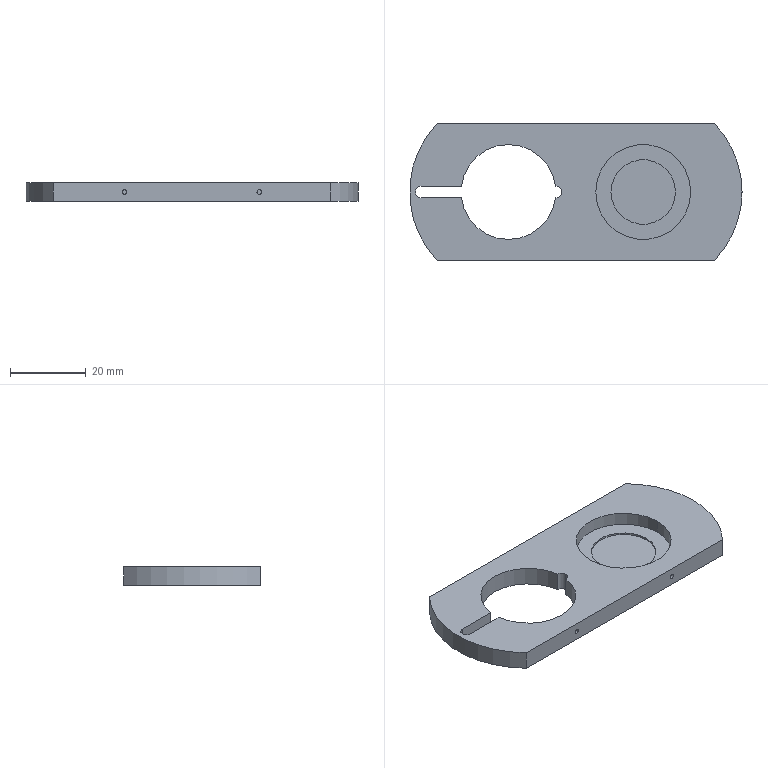Part | STEP file | TCHK-2D-D30-BB-2.stp.STEP | 1 solid | 28 faces | box 87.5 x 36 x 5 mm | volume 10454 mm3 | cylinder 16 | plane 12 | commonest cylinder face diameters 1.2 x4 25 x4 3 x3 52 x3 17 x2
STEP:
#1=CARTESIAN_POINT('',(-5.34,1.5,-2.5));
#2=VERTEX_POINT('',#1);
#3=CARTESIAN_POINT('',(-30.16,1.5,-2.5));
#4=VERTEX_POINT('',#3);
#5=CARTESIAN_POINT('',(-17.75,0.,-2.5));
#6=DIRECTION('',(0.,0.,1.));
#7=DIRECTION('',(0.9928,0.12,0.));
#8=AXIS2_PLACEMENT_3D('',#5,#6,#7);
#9=CIRCLE('',#8,12.5);
#10=EDGE_CURVE('',#2,#4,#9,.T.);
#11=ORIENTED_EDGE('',*,*,#10,.T.);
#12=CARTESIAN_POINT('',(-40.75,1.5,-2.5));
#13=VERTEX_POINT('',#12);
#14=CARTESIAN_POINT('',(-30.16,1.5,-2.5));
#15=DIRECTION('',(-1.,0.,0.));
#16=VECTOR('',#15,1000.);
#17=LINE('',#14,#16);
#18=EDGE_CURVE('',#4,#13,#17,.T.);
#19=ORIENTED_EDGE('',*,*,#18,.T.);
#20=CARTESIAN_POINT('',(-40.75,-1.5,-2.5));
#21=VERTEX_POINT('',#20);
#22=CARTESIAN_POINT('',(-40.75,0.,-2.5));
#23=DIRECTION('',(0.,0.,1.));
#24=DIRECTION('',(0.,1.,0.));
#25=AXIS2_PLACEMENT_3D('',#22,#23,#24);
#26=CIRCLE('',#25,1.5);
#27=EDGE_CURVE('',#13,#21,#26,.T.);
#28=ORIENTED_EDGE('',*,*,#27,.T.);
#29=CARTESIAN_POINT('',(-30.16,-1.5,-2.5));
#30=VERTEX_POINT('',#29);
#31=CARTESIAN_POINT('',(-40.75,-1.5,-2.5));
#32=DIRECTION('',(1.,0.,0.));
#33=VECTOR('',#32,1000.);
#34=LINE('',#31,#33);
#35=EDGE_CURVE('',#21,#30,#34,.T.);
#36=ORIENTED_EDGE('',*,*,#35,.T.);
#37=CARTESIAN_POINT('',(-5.34,-1.5,-2.5));
#38=VERTEX_POINT('',#37);
#39=CARTESIAN_POINT('',(-17.75,0.,-2.5));
#40=DIRECTION('',(0.,0.,1.));
#41=DIRECTION('',(-0.9928,-0.12,0.));
#42=AXIS2_PLACEMENT_3D('',#39,#40,#41);
#43=CIRCLE('',#42,12.5);
#44=EDGE_CURVE('',#30,#38,#43,.T.);
#45=ORIENTED_EDGE('',*,*,#44,.T.);
#46=CARTESIAN_POINT('',(-5.25,-1.5,-2.5));
#47=VERTEX_POINT('',#46);
#48=CARTESIAN_POINT('',(-5.34,-1.5,-2.5));
#49=DIRECTION('',(1.,0.,0.));
#50=VECTOR('',#49,1000.);
#51=LINE('',#48,#50);
#52=EDGE_CURVE('',#38,#47,#51,.T.);
#53=ORIENTED_EDGE('',*,*,#52,.T.);
#54=CARTESIAN_POINT('',(-3.75,0.,-2.5));
#55=VERTEX_POINT('',#54);
#56=CARTESIAN_POINT('',(-5.25,0.,-2.5));
#57=DIRECTION('',(0.,0.,1.));
#58=DIRECTION('',(0.,-1.,0.));
#59=AXIS2_PLACEMENT_3D('',#56,#57,#58);
#60=CIRCLE('',#59,1.5);
#61=EDGE_CURVE('',#47,#55,#60,.T.);
#62=ORIENTED_EDGE('',*,*,#61,.T.);
#63=CARTESIAN_POINT('',(-5.25,1.5,-2.5));
#64=VERTEX_POINT('',#63);
#65=CARTESIAN_POINT('',(-5.25,0.,-2.5));
#66=DIRECTION('',(0.,0.,1.));
#67=DIRECTION('',(0.,-1.,0.));
#68=AXIS2_PLACEMENT_3D('',#65,#66,#67);
#69=CIRCLE('',#68,1.5);
#70=EDGE_CURVE('',#55,#64,#69,.T.);
#71=ORIENTED_EDGE('',*,*,#70,.T.);
#72=CARTESIAN_POINT('',(-5.25,1.5,-2.5));
#73=DIRECTION('',(-1.,0.,0.));
#74=VECTOR('',#73,1000.);
#75=LINE('',#72,#74);
#76=EDGE_CURVE('',#64,#2,#75,.T.);
#77=ORIENTED_EDGE('',*,*,#76,.T.);
#78=EDGE_LOOP('',(#11,#19,#28,#36,#45,#53,#62,#71,#77));
#79=FACE_BOUND('',#78,.T.);
#80=CARTESIAN_POINT('',(36.512,18.,-2.5));
#81=VERTEX_POINT('',#80);
#82=CARTESIAN_POINT('',(-36.512,18.,-2.5));
#83=VERTEX_POINT('',#82);
#84=CARTESIAN_POINT('',(36.512,18.,-2.5));
#85=DIRECTION('',(-1.,0.,0.));
#86=VECTOR('',#85,1000.);
#87=LINE('',#84,#86);
#88=EDGE_CURVE('',#81,#83,#87,.T.);
#89=ORIENTED_EDGE('',*,*,#88,.F.);
#90=CARTESIAN_POINT('',(43.75,0.,-2.5));
#91=VERTEX_POINT('',#90);
#92=CARTESIAN_POINT('',(17.75,0.,-2.5));
#93=DIRECTION('',(0.,0.,1.));
#94=DIRECTION('',(0.7216,-0.6923,0.));
#95=AXIS2_PLACEMENT_3D('',#92,#93,#94);
#96=CIRCLE('',#95,26.);
#97=EDGE_CURVE('',#91,#81,#96,.T.);
#98=ORIENTED_EDGE('',*,*,#97,.F.);
#99=CARTESIAN_POINT('',(36.512,-18.,-2.5));
#100=VERTEX_POINT('',#99);
#101=CARTESIAN_POINT('',(17.75,0.,-2.5));
#102=DIRECTION('',(0.,0.,1.));
#103=DIRECTION('',(0.7216,-0.6923,0.));
#104=AXIS2_PLACEMENT_3D('',#101,#102,#103);
#105=CIRCLE('',#104,26.);
#106=EDGE_CURVE('',#100,#91,#105,.T.);
#107=ORIENTED_EDGE('',*,*,#106,.F.);
#108=CARTESIAN_POINT('',(-36.512,-18.,-2.5));
#109=VERTEX_POINT('',#108);
#110=CARTESIAN_POINT('',(-36.512,-18.,-2.5));
#111=DIRECTION('',(1.,0.,0.));
#112=VECTOR('',#111,1000.);
#113=LINE('',#110,#112);
#114=EDGE_CURVE('',#109,#100,#113,.T.);
#115=ORIENTED_EDGE('',*,*,#114,.F.);
#116=CARTESIAN_POINT('',(-17.75,0.,-2.5));
#117=DIRECTION('',(0.,0.,1.));
#118=DIRECTION('',(-0.7216,0.6923,0.));
#119=AXIS2_PLACEMENT_3D('',#116,#117,#118);
#120=CIRCLE('',#119,26.);
#121=EDGE_CURVE('',#83,#109,#120,.T.);
#122=ORIENTED_EDGE('',*,*,#121,.F.);
#123=EDGE_LOOP('',(#89,#98,#107,#115,#122));
#124=FACE_OUTER_BOUND('',#123,.T.);
#125=CARTESIAN_POINT('',(0.,0.,-2.5));
#126=DIRECTION('',(0.,0.,1.));
#127=DIRECTION('',(1.,0.,0.));
#128=AXIS2_PLACEMENT_3D('',#125,#126,#127);
#129=PLANE('',#128);
#130=ADVANCED_FACE('',(#79,#124),#129,.F.);
#131=CARTESIAN_POINT('',(-36.512,-18.,2.5));
#132=VERTEX_POINT('',#131);
#133=CARTESIAN_POINT('',(-36.512,-18.,-2.5));
#134=DIRECTION('',(0.,0.,1.));
#135=VECTOR('',#134,1000.);
#136=LINE('',#133,#135);
#137=EDGE_CURVE('',#109,#132,#136,.T.);
#138=ORIENTED_EDGE('',*,*,#137,.T.);
#139=CARTESIAN_POINT('',(-36.512,18.,2.5));
#140=VERTEX_POINT('',#139);
#141=CARTESIAN_POINT('',(-17.75,0.,2.5));
#142=DIRECTION('',(0.,0.,1.));
#143=DIRECTION('',(-0.7216,0.6923,0.));
#144=AXIS2_PLACEMENT_3D('',#141,#142,#143);
#145=CIRCLE('',#144,26.);
#146=EDGE_CURVE('',#140,#132,#145,.T.);
#147=ORIENTED_EDGE('',*,*,#146,.F.);
#148=CARTESIAN_POINT('',(-36.512,18.,-2.5));
#149=DIRECTION('',(0.,0.,1.));
#150=VECTOR('',#149,1000.);
#151=LINE('',#148,#150);
#152=EDGE_CURVE('',#83,#140,#151,.T.);
#153=ORIENTED_EDGE('',*,*,#152,.F.);
#154=ORIENTED_EDGE('',*,*,#121,.T.);
#155=EDGE_LOOP('',(#138,#147,#153,#154));
#156=FACE_OUTER_BOUND('',#155,.T.);
#157=CARTESIAN_POINT('',(-17.75,0.,-2.5));
#158=DIRECTION('',(0.,0.,1.));
#159=DIRECTION('',(1.,0.,0.));
#160=AXIS2_PLACEMENT_3D('',#157,#158,#159);
#161=CYLINDRICAL_SURFACE('',#160,26.);
#162=ADVANCED_FACE('',(#156),#161,.T.);
#163=ORIENTED_EDGE('',*,*,#152,.T.);
#164=CARTESIAN_POINT('',(36.512,18.,2.5));
#165=VERTEX_POINT('',#164);
#166=CARTESIAN_POINT('',(36.512,18.,2.5));
#167=DIRECTION('',(-1.,0.,0.));
#168=VECTOR('',#167,1000.);
#169=LINE('',#166,#168);
#170=EDGE_CURVE('',#165,#140,#169,.T.);
#171=ORIENTED_EDGE('',*,*,#170,.F.);
#172=CARTESIAN_POINT('',(36.512,18.,-2.5));
#173=DIRECTION('',(0.,0.,1.));
#174=VECTOR('',#173,1000.);
#175=LINE('',#172,#174);
#176=EDGE_CURVE('',#81,#165,#175,.T.);
#177=ORIENTED_EDGE('',*,*,#176,.F.);
#178=ORIENTED_EDGE('',*,*,#88,.T.);
#179=EDGE_LOOP('',(#163,#171,#177,#178));
#180=FACE_OUTER_BOUND('',#179,.T.);
#181=CARTESIAN_POINT('',(36.512,18.,-2.5));
#182=DIRECTION('',(0.,1.,0.));
#183=DIRECTION('',(1.,0.,0.));
#184=AXIS2_PLACEMENT_3D('',#181,#182,#183);
#185=PLANE('',#184);
#186=ADVANCED_FACE('',(#180),#185,.T.);
#187=CARTESIAN_POINT('',(43.75,0.,2.5));
#188=VERTEX_POINT('',#187);
#189=CARTESIAN_POINT('',(43.75,0.,-2.5));
#190=DIRECTION('',(0.,0.,1.));
#191=VECTOR('',#190,1000.);
#192=LINE('',#189,#191);
#193=EDGE_CURVE('',#91,#188,#192,.T.);
#194=ORIENTED_EDGE('',*,*,#193,.F.);
#195=ORIENTED_EDGE('',*,*,#97,.T.);
#196=ORIENTED_EDGE('',*,*,#176,.T.);
#197=CARTESIAN_POINT('',(17.75,0.,2.5));
#198=DIRECTION('',(0.,0.,1.));
#199=DIRECTION('',(0.7216,-0.6923,0.));
#200=AXIS2_PLACEMENT_3D('',#197,#198,#199);
#201=CIRCLE('',#200,26.);
#202=EDGE_CURVE('',#188,#165,#201,.T.);
#203=ORIENTED_EDGE('',*,*,#202,.F.);
#204=EDGE_LOOP('',(#194,#195,#196,#203));
#205=FACE_OUTER_BOUND('',#204,.T.);
#206=CARTESIAN_POINT('',(17.75,0.,-2.5));
#207=DIRECTION('',(0.,0.,1.));
#208=DIRECTION('',(1.,0.,0.));
#209=AXIS2_PLACEMENT_3D('',#206,#207,#208);
#210=CYLINDRICAL_SURFACE('',#209,26.);
#211=ADVANCED_FACE('',(#205),#210,.T.);
#212=CARTESIAN_POINT('',(-18.35,-18.,0.));
#213=VERTEX_POINT('',#212);
#214=CARTESIAN_POINT('',(-17.15,-18.,0.));
#215=VERTEX_POINT('',#214);
#216=CARTESIAN_POINT('',(-17.75,-18.,0.));
#217=DIRECTION('',(0.,1.,0.));
#218=DIRECTION('',(-1.,0.,0.));
#219=AXIS2_PLACEMENT_3D('',#216,#217,#218);
#220=CIRCLE('',#219,0.6);
#221=EDGE_CURVE('',#213,#215,#220,.T.);
#222=ORIENTED_EDGE('',*,*,#221,.T.);
#223=CARTESIAN_POINT('',(-17.75,-18.,0.));
#224=DIRECTION('',(0.,1.,0.));
#225=DIRECTION('',(1.,0.,0.));
#226=AXIS2_PLACEMENT_3D('',#223,#224,#225);
#227=CIRCLE('',#226,0.6);
#228=EDGE_CURVE('',#215,#213,#227,.T.);
#229=ORIENTED_EDGE('',*,*,#228,.T.);
#230=EDGE_LOOP('',(#222,#229));
#231=FACE_BOUND('',#230,.T.);
#232=CARTESIAN_POINT('',(17.15,-18.,0.));
#233=VERTEX_POINT('',#232);
#234=CARTESIAN_POINT('',(18.35,-18.,0.));
#235=VERTEX_POINT('',#234);
#236=CARTESIAN_POINT('',(17.75,-18.,0.));
#237=DIRECTION('',(0.,1.,0.));
#238=DIRECTION('',(-1.,0.,0.));
#239=AXIS2_PLACEMENT_3D('',#236,#237,#238);
#240=CIRCLE('',#239,0.6);
#241=EDGE_CURVE('',#233,#235,#240,.T.);
#242=ORIENTED_EDGE('',*,*,#241,.T.);
#243=CARTESIAN_POINT('',(17.75,-18.,0.));
#244=DIRECTION('',(0.,1.,0.));
#245=DIRECTION('',(1.,0.,0.));
#246=AXIS2_PLACEMENT_3D('',#243,#244,#245);
#247=CIRCLE('',#246,0.6);
#248=EDGE_CURVE('',#235,#233,#247,.T.);
#249=ORIENTED_EDGE('',*,*,#248,.T.);
#250=EDGE_LOOP('',(#242,#249));
#251=FACE_BOUND('',#250,.T.);
#252=CARTESIAN_POINT('',(36.512,-18.,2.5));
#253=VERTEX_POINT('',#252);
#254=CARTESIAN_POINT('',(36.512,-18.,-2.5));
#255=DIRECTION('',(0.,0.,1.));
#256=VECTOR('',#255,1000.);
#257=LINE('',#254,#256);
#258=EDGE_CURVE('',#100,#253,#257,.T.);
#259=ORIENTED_EDGE('',*,*,#258,.T.);
#260=CARTESIAN_POINT('',(-36.512,-18.,2.5));
#261=DIRECTION('',(1.,0.,0.));
#262=VECTOR('',#261,1000.);
#263=LINE('',#260,#262);
#264=EDGE_CURVE('',#132,#253,#263,.T.);
#265=ORIENTED_EDGE('',*,*,#264,.F.);
#266=ORIENTED_EDGE('',*,*,#137,.F.);
#267=ORIENTED_EDGE('',*,*,#114,.T.);
#268=EDGE_LOOP('',(#259,#265,#266,#267));
#269=FACE_OUTER_BOUND('',#268,.T.);
#270=CARTESIAN_POINT('',(-36.512,-18.,-2.5));
#271=DIRECTION('',(0.,-1.,0.));
#272=DIRECTION('',(0.,0.,-1.));
#273=AXIS2_PLACEMENT_3D('',#270,#271,#272);
#274=PLANE('',#273);
#275=ADVANCED_FACE('',(#231,#251,#269),#274,.T.);
#276=CARTESIAN_POINT('',(5.25,0.,2.5));
#277=VERTEX_POINT('',#276);
#278=CARTESIAN_POINT('',(30.25,0.,2.5));
#279=VERTEX_POINT('',#278);
#280=CARTESIAN_POINT('',(17.75,0.,2.5));
#281=DIRECTION('',(0.,0.,1.));
#282=DIRECTION('',(-1.,0.,0.));
#283=AXIS2_PLACEMENT_3D('',#280,#281,#282);
#284=CIRCLE('',#283,12.5);
#285=EDGE_CURVE('',#277,#279,#284,.T.);
#286=ORIENTED_EDGE('',*,*,#285,.F.);
#287=CARTESIAN_POINT('',(17.75,0.,2.5));
#288=DIRECTION('',(0.,0.,1.));
#289=DIRECTION('',(1.,0.,0.));
#290=AXIS2_PLACEMENT_3D('',#287,#288,#289);
#291=CIRCLE('',#290,12.5);
#292=EDGE_CURVE('',#279,#277,#291,.T.);
#293=ORIENTED_EDGE('',*,*,#292,.F.);
#294=EDGE_LOOP('',(#286,#293));
#295=FACE_BOUND('',#294,.T.);
#296=CARTESIAN_POINT('',(-5.25,-1.5,2.5));
#297=VERTEX_POINT('',#296);
#298=CARTESIAN_POINT('',(-3.75,0.,2.5));
#299=VERTEX_POINT('',#298);
#300=CARTESIAN_POINT('',(-5.25,0.,2.5));
#301=DIRECTION('',(0.,0.,1.));
#302=DIRECTION('',(0.,-1.,0.));
#303=AXIS2_PLACEMENT_3D('',#300,#301,#302);
#304=CIRCLE('',#303,1.5);
#305=EDGE_CURVE('',#297,#299,#304,.T.);
#306=ORIENTED_EDGE('',*,*,#305,.F.);
#307=CARTESIAN_POINT('',(-5.34,-1.5,2.5));
#308=VERTEX_POINT('',#307);
#309=CARTESIAN_POINT('',(-5.34,-1.5,2.5));
#310=DIRECTION('',(1.,0.,0.));
#311=VECTOR('',#310,1000.);
#312=LINE('',#309,#311);
#313=EDGE_CURVE('',#308,#297,#312,.T.);
#314=ORIENTED_EDGE('',*,*,#313,.F.);
#315=CARTESIAN_POINT('',(-30.16,-1.5,2.5));
#316=VERTEX_POINT('',#315);
#317=CARTESIAN_POINT('',(-17.75,0.,2.5));
#318=DIRECTION('',(0.,0.,1.));
#319=DIRECTION('',(-0.9928,-0.12,0.));
#320=AXIS2_PLACEMENT_3D('',#317,#318,#319);
#321=CIRCLE('',#320,12.5);
#322=EDGE_CURVE('',#316,#308,#321,.T.);
#323=ORIENTED_EDGE('',*,*,#322,.F.);
#324=CARTESIAN_POINT('',(-40.75,-1.5,2.5));
#325=VERTEX_POINT('',#324);
#326=CARTESIAN_POINT('',(-40.75,-1.5,2.5));
#327=DIRECTION('',(1.,0.,0.));
#328=VECTOR('',#327,1000.);
#329=LINE('',#326,#328);
#330=EDGE_CURVE('',#325,#316,#329,.T.);
#331=ORIENTED_EDGE('',*,*,#330,.F.);
#332=CARTESIAN_POINT('',(-40.75,1.5,2.5));
#333=VERTEX_POINT('',#332);
#334=CARTESIAN_POINT('',(-40.75,0.,2.5));
#335=DIRECTION('',(0.,0.,1.));
#336=DIRECTION('',(0.,1.,0.));
#337=AXIS2_PLACEMENT_3D('',#334,#335,#336);
#338=CIRCLE('',#337,1.5);
#339=EDGE_CURVE('',#333,#325,#338,.T.);
#340=ORIENTED_EDGE('',*,*,#339,.F.);
#341=CARTESIAN_POINT('',(-30.16,1.5,2.5));
#342=VERTEX_POINT('',#341);
#343=CARTESIAN_POINT('',(-30.16,1.5,2.5));
#344=DIRECTION('',(-1.,0.,0.));
#345=VECTOR('',#344,1000.);
#346=LINE('',#343,#345);
#347=EDGE_CURVE('',#342,#333,#346,.T.);
#348=ORIENTED_EDGE('',*,*,#347,.F.);
#349=CARTESIAN_POINT('',(-5.34,1.5,2.5));
#350=VERTEX_POINT('',#349);
#351=CARTESIAN_POINT('',(-17.75,0.,2.5));
#352=DIRECTION('',(0.,0.,1.));
#353=DIRECTION('',(0.9928,0.12,0.));
#354=AXIS2_PLACEMENT_3D('',#351,#352,#353);
#355=CIRCLE('',#354,12.5);
#356=EDGE_CURVE('',#350,#342,#355,.T.);
#357=ORIENTED_EDGE('',*,*,#356,.F.);
#358=CARTESIAN_POINT('',(-5.25,1.5,2.5));
#359=VERTEX_POINT('',#358);
#360=CARTESIAN_POINT('',(-5.25,1.5,2.5));
#361=DIRECTION('',(-1.,0.,0.));
#362=VECTOR('',#361,1000.);
#363=LINE('',#360,#362);
#364=EDGE_CURVE('',#359,#350,#363,.T.);
#365=ORIENTED_EDGE('',*,*,#364,.F.);
#366=CARTESIAN_POINT('',(-5.25,0.,2.5));
#367=DIRECTION('',(0.,0.,1.));
#368=DIRECTION('',(0.,-1.,0.));
#369=AXIS2_PLACEMENT_3D('',#366,#367,#368);
#370=CIRCLE('',#369,1.5);
#371=EDGE_CURVE('',#299,#359,#370,.T.);
#372=ORIENTED_EDGE('',*,*,#371,.F.);
#373=EDGE_LOOP('',(#306,#314,#323,#331,#340,#348,#357,#365,#372));
#374=FACE_BOUND('',#373,.T.);
#375=ORIENTED_EDGE('',*,*,#264,.T.);
#376=CARTESIAN_POINT('',(17.75,0.,2.5));
#377=DIRECTION('',(0.,0.,1.));
#378=DIRECTION('',(0.7216,-0.6923,0.));
#379=AXIS2_PLACEMENT_3D('',#376,#377,#378);
#380=CIRCLE('',#379,26.);
#381=EDGE_CURVE('',#253,#188,#380,.T.);
#382=ORIENTED_EDGE('',*,*,#381,.T.);
#383=ORIENTED_EDGE('',*,*,#202,.T.);
#384=ORIENTED_EDGE('',*,*,#170,.T.);
#385=ORIENTED_EDGE('',*,*,#146,.T.);
#386=EDGE_LOOP('',(#375,#382,#383,#384,#385));
#387=FACE_OUTER_BOUND('',#386,.T.);
#388=CARTESIAN_POINT('',(0.,0.,2.5));
#389=DIRECTION('',(0.,0.,1.));
#390=DIRECTION('',(1.,0.,0.));
#391=AXIS2_PLACEMENT_3D('',#388,#389,#390);
#392=PLANE('',#391);
#393=ADVANCED_FACE('',(#295,#374,#387),#392,.T.);
#394=CARTESIAN_POINT('',(5.25,0.,-1.));
#395=VERTEX_POINT('',#394);
#396=CARTESIAN_POINT('',(5.25,0.,2.5));
#397=DIRECTION('',(0.,0.,-1.));
#398=VECTOR('',#397,1000.);
#399=LINE('',#396,#398);
#400=EDGE_CURVE('',#277,#395,#399,.T.);
#401=ORIENTED_EDGE('',*,*,#400,.T.);
#402=CARTESIAN_POINT('',(30.25,0.,-1.));
#403=VERTEX_POINT('',#402);
#404=CARTESIAN_POINT('',(17.75,0.,-1.));
#405=DIRECTION('',(0.,0.,-1.));
#406=DIRECTION('',(-1.,0.,0.));
#407=AXIS2_PLACEMENT_3D('',#404,#405,#406);
#408=CIRCLE('',#407,12.5);
#409=EDGE_CURVE('',#395,#403,#408,.T.);
#410=ORIENTED_EDGE('',*,*,#409,.T.);
#411=CARTESIAN_POINT('',(30.25,0.,2.5));
#412=DIRECTION('',(0.,0.,-1.));
#413=VECTOR('',#412,1000.);
#414=LINE('',#411,#413);
#415=EDGE_CURVE('',#279,#403,#414,.T.);
#416=ORIENTED_EDGE('',*,*,#415,.F.);
#417=ORIENTED_EDGE('',*,*,#292,.T.);
#418=EDGE_LOOP('',(#401,#410,#416,#417));
#419=FACE_OUTER_BOUND('',#418,.T.);
#420=CARTESIAN_POINT('',(17.75,0.,2.5));
#421=DIRECTION('',(0.,0.,1.));
#422=DIRECTION('',(1.,0.,0.));
#423=AXIS2_PLACEMENT_3D('',#420,#421,#422);
#424=CYLINDRICAL_SURFACE('',#423,12.5);
#425=ADVANCED_FACE('',(#419),#424,.F.);
#426=ORIENTED_EDGE('',*,*,#415,.T.);
#427=CARTESIAN_POINT('',(17.75,0.,-1.));
#428=DIRECTION('',(0.,0.,-1.));
#429=DIRECTION('',(1.,0.,0.));
#430=AXIS2_PLACEMENT_3D('',#427,#428,#429);
#431=CIRCLE('',#430,12.5);
#432=EDGE_CURVE('',#403,#395,#431,.T.);
#433=ORIENTED_EDGE('',*,*,#432,.T.);
#434=ORIENTED_EDGE('',*,*,#400,.F.);
#435=ORIENTED_EDGE('',*,*,#285,.T.);
#436=EDGE_LOOP('',(#426,#433,#434,#435));
#437=FACE_OUTER_BOUND('',#436,.T.);
#438=CARTESIAN_POINT('',(17.75,0.,2.5));
#439=DIRECTION('',(0.,0.,1.));
#440=DIRECTION('',(1.,0.,0.));
#441=AXIS2_PLACEMENT_3D('',#438,#439,#440);
#442=CYLINDRICAL_SURFACE('',#441,12.5);
#443=ADVANCED_FACE('',(#437),#442,.F.);
#444=CARTESIAN_POINT('',(9.25,0.,-1.));
#445=VERTEX_POINT('',#444);
#446=CARTESIAN_POINT('',(26.25,0.,-1.));
#447=VERTEX_POINT('',#446);
#448=CARTESIAN_POINT('',(17.75,0.,-1.));
#449=DIRECTION('',(0.,0.,1.));
#450=DIRECTION('',(-1.,0.,0.));
#451=AXIS2_PLACEMENT_3D('',#448,#449,#450);
#452=CIRCLE('',#451,8.5);
#453=EDGE_CURVE('',#445,#447,#452,.T.);
#454=ORIENTED_EDGE('',*,*,#453,.F.);
#455=CARTESIAN_POINT('',(17.75,0.,-1.));
#456=DIRECTION('',(0.,0.,1.));
#457=DIRECTION('',(1.,0.,0.));
#458=AXIS2_PLACEMENT_3D('',#455,#456,#457);
#459=CIRCLE('',#458,8.5);
#460=EDGE_CURVE('',#447,#445,#459,.T.);
#461=ORIENTED_EDGE('',*,*,#460,.F.);
#462=EDGE_LOOP('',(#454,#461));
#463=FACE_BOUND('',#462,.T.);
#464=ORIENTED_EDGE('',*,*,#432,.F.);
#465=ORIENTED_EDGE('',*,*,#409,.F.);
#466=EDGE_LOOP('',(#464,#465));
#467=FACE_OUTER_BOUND('',#466,.T.);
#468=CARTESIAN_POINT('',(0.,0.,-1.));
#469=DIRECTION('',(0.,0.,1.));
#470=DIRECTION('',(1.,0.,0.));
#471=AXIS2_PLACEMENT_3D('',#468,#469,#470);
#472=PLANE('',#471);
#473=ADVANCED_FACE('',(#463,#467),#472,.T.);
#474=CARTESIAN_POINT('',(9.25,0.,-1.5));
#475=VERTEX_POINT('',#474);
#476=CARTESIAN_POINT('',(9.25,0.,-1.));
#477=DIRECTION('',(0.,0.,-1.));
#478=VECTOR('',#477,1000.);
#479=LINE('',#476,#478);
#480=EDGE_CURVE('',#445,#475,#479,.T.);
#481=ORIENTED_EDGE('',*,*,#480,.T.);
#482=CARTESIAN_POINT('',(26.25,0.,-1.5));
#483=VERTEX_POINT('',#482);
#484=CARTESIAN_POINT('',(17.75,0.,-1.5));
#485=DIRECTION('',(0.,0.,1.));
#486=DIRECTION('',(1.,0.,0.));
#487=AXIS2_PLACEMENT_3D('',#484,#485,#486);
#488=CIRCLE('',#487,8.5);
#489=EDGE_CURVE('',#483,#475,#488,.T.);
#490=ORIENTED_EDGE('',*,*,#489,.F.);
#491=CARTESIAN_POINT('',(26.25,0.,-1.));
#492=DIRECTION('',(0.,0.,-1.));
#493=VECTOR('',#492,1000.);
#494=LINE('',#491,#493);
#495=EDGE_CURVE('',#447,#483,#494,.T.);
#496=ORIENTED_EDGE('',*,*,#495,.F.);
#497=ORIENTED_EDGE('',*,*,#460,.T.);
#498=EDGE_LOOP('',(#481,#490,#496,#497));
#499=FACE_OUTER_BOUND('',#498,.T.);
#500=CARTESIAN_POINT('',(17.75,0.,-1.));
#501=DIRECTION('',(0.,0.,1.));
#502=DIRECTION('',(1.,0.,0.));
#503=AXIS2_PLACEMENT_3D('',#500,#501,#502);
#504=CYLINDRICAL_SURFACE('',#503,8.5);
#505=ADVANCED_FACE('',(#499),#504,.F.);
#506=ORIENTED_EDGE('',*,*,#495,.T.);
#507=CARTESIAN_POINT('',(17.75,0.,-1.5));
#508=DIRECTION('',(0.,0.,1.));
#509=DIRECTION('',(-1.,0.,0.));
#510=AXIS2_PLACEMENT_3D('',#507,#508,#509);
#511=CIRCLE('',#510,8.5);
#512=EDGE_CURVE('',#475,#483,#511,.T.);
#513=ORIENTED_EDGE('',*,*,#512,.F.);
#514=ORIENTED_EDGE('',*,*,#480,.F.);
#515=ORIENTED_EDGE('',*,*,#453,.T.);
#516=EDGE_LOOP('',(#506,#513,#514,#515));
#517=FACE_OUTER_BOUND('',#516,.T.);
#518=CARTESIAN_POINT('',(17.75,0.,-1.));
#519=DIRECTION('',(0.,0.,1.));
#520=DIRECTION('',(1.,0.,0.));
#521=AXIS2_PLACEMENT_3D('',#518,#519,#520);
#522=CYLINDRICAL_SURFACE('',#521,8.5);
#523=ADVANCED_FACE('',(#517),#522,.F.);
#524=ORIENTED_EDGE('',*,*,#512,.T.);
#525=ORIENTED_EDGE('',*,*,#489,.T.);
#526=EDGE_LOOP('',(#524,#525));
#527=FACE_OUTER_BOUND('',#526,.T.);
#528=CARTESIAN_POINT('',(0.,0.,-1.5));
#529=DIRECTION('',(0.,0.,1.));
#530=DIRECTION('',(1.,0.,0.));
#531=AXIS2_PLACEMENT_3D('',#528,#529,#530);
#532=PLANE('',#531);
#533=ADVANCED_FACE('',(#527),#532,.T.);
#534=CARTESIAN_POINT('',(-5.25,1.5,2.5));
#535=DIRECTION('',(0.,0.,-1.));
#536=VECTOR('',#535,1000.);
#537=LINE('',#534,#536);
#538=EDGE_CURVE('',#359,#64,#537,.T.);
#539=ORIENTED_EDGE('',*,*,#538,.F.);
#540=ORIENTED_EDGE('',*,*,#364,.T.);
#541=CARTESIAN_POINT('',(-5.34,1.5,-2.5));
#542=DIRECTION('',(0.,0.,1.));
#543=VECTOR('',#542,1000.);
#544=LINE('',#541,#543);
#545=EDGE_CURVE('',#2,#350,#544,.T.);
#546=ORIENTED_EDGE('',*,*,#545,.F.);
#547=ORIENTED_EDGE('',*,*,#76,.F.);
#548=EDGE_LOOP('',(#539,#540,#546,#547));
#549=FACE_OUTER_BOUND('',#548,.T.);
#550=CARTESIAN_POINT('',(-5.25,1.5,2.5));
#551=DIRECTION('',(0.,1.,0.));
#552=DIRECTION('',(1.,0.,0.));
#553=AXIS2_PLACEMENT_3D('',#550,#551,#552);
#554=PLANE('',#553);
#555=ADVANCED_FACE('',(#549),#554,.F.);
#556=CARTESIAN_POINT('',(-30.16,1.5,-2.5));
#557=DIRECTION('',(0.,0.,1.));
#558=VECTOR('',#557,1000.);
#559=LINE('',#556,#558);
#560=EDGE_CURVE('',#4,#342,#559,.T.);
#561=ORIENTED_EDGE('',*,*,#560,.T.);
#562=ORIENTED_EDGE('',*,*,#347,.T.);
#563=CARTESIAN_POINT('',(-40.75,1.5,2.5));
#564=DIRECTION('',(0.,0.,-1.));
#565=VECTOR('',#564,1000.);
#566=LINE('',#563,#565);
#567=EDGE_CURVE('',#333,#13,#566,.T.);
#568=ORIENTED_EDGE('',*,*,#567,.T.);
#569=ORIENTED_EDGE('',*,*,#18,.F.);
#570=EDGE_LOOP('',(#561,#562,#568,#569));
#571=FACE_OUTER_BOUND('',#570,.T.);
#572=CARTESIAN_POINT('',(-5.25,1.5,2.5));
#573=DIRECTION('',(0.,1.,0.));
#574=DIRECTION('',(1.,0.,0.));
#575=AXIS2_PLACEMENT_3D('',#572,#573,#574);
#576=PLANE('',#575);
#577=ADVANCED_FACE('',(#571),#576,.F.);
#578=ORIENTED_EDGE('',*,*,#356,.T.);
#579=ORIENTED_EDGE('',*,*,#560,.F.);
#580=ORIENTED_EDGE('',*,*,#10,.F.);
#581=ORIENTED_EDGE('',*,*,#545,.T.);
#582=EDGE_LOOP('',(#578,#579,#580,#581));
#583=FACE_OUTER_BOUND('',#582,.T.);
#584=CARTESIAN_POINT('',(-17.75,0.,2.5));
#585=DIRECTION('',(0.,0.,1.));
#586=DIRECTION('',(1.,0.,0.));
#587=AXIS2_PLACEMENT_3D('',#584,#585,#586);
#588=CYLINDRICAL_SURFACE('',#587,12.5);
#589=ADVANCED_FACE('',(#583),#588,.F.);
#590=CARTESIAN_POINT('',(-3.75,0.,2.5));
#591=DIRECTION('',(0.,0.,1.));
#592=VECTOR('',#591,1000.);
#593=LINE('',#590,#592);
#594=EDGE_CURVE('',#55,#299,#593,.T.);
#595=ORIENTED_EDGE('',*,*,#594,.F.);
#596=ORIENTED_EDGE('',*,*,#61,.F.);
#597=CARTESIAN_POINT('',(-5.25,-1.5,2.5));
#598=DIRECTION('',(0.,0.,-1.));
#599=VECTOR('',#598,1000.);
#600=LINE('',#597,#599);
#601=EDGE_CURVE('',#297,#47,#600,.T.);
#602=ORIENTED_EDGE('',*,*,#601,.F.);
#603=ORIENTED_EDGE('',*,*,#305,.T.);
#604=EDGE_LOOP('',(#595,#596,#602,#603));
#605=FACE_OUTER_BOUND('',#604,.T.);
#606=CARTESIAN_POINT('',(-5.25,0.,2.5));
#607=DIRECTION('',(0.,0.,1.));
#608=DIRECTION('',(1.,0.,0.));
#609=AXIS2_PLACEMENT_3D('',#606,#607,#608);
#610=CYLINDRICAL_SURFACE('',#609,1.5);
#611=ADVANCED_FACE('',(#605),#610,.F.);
#612=CARTESIAN_POINT('',(-40.75,-1.5,2.5));
#613=DIRECTION('',(0.,0.,-1.));
#614=VECTOR('',#613,1000.);
#615=LINE('',#612,#614);
#616=EDGE_CURVE('',#325,#21,#615,.T.);
#617=ORIENTED_EDGE('',*,*,#616,.F.);
#618=ORIENTED_EDGE('',*,*,#330,.T.);
#619=CARTESIAN_POINT('',(-30.16,-1.5,-2.5));
#620=DIRECTION('',(0.,0.,1.));
#621=VECTOR('',#620,1000.);
#622=LINE('',#619,#621);
#623=EDGE_CURVE('',#30,#316,#622,.T.);
#624=ORIENTED_EDGE('',*,*,#623,.F.);
#625=ORIENTED_EDGE('',*,*,#35,.F.);
#626=EDGE_LOOP('',(#617,#618,#624,#625));
#627=FACE_OUTER_BOUND('',#626,.T.);
#628=CARTESIAN_POINT('',(-40.75,-1.5,2.5));
#629=DIRECTION('',(0.,-1.,0.));
#630=DIRECTION('',(0.,0.,-1.));
#631=AXIS2_PLACEMENT_3D('',#628,#629,#630);
#632=PLANE('',#631);
#633=ADVANCED_FACE('',(#627),#632,.F.);
#634=CARTESIAN_POINT('',(-5.34,-1.5,-2.5));
#635=DIRECTION('',(0.,0.,1.));
#636=VECTOR('',#635,1000.);
#637=LINE('',#634,#636);
#638=EDGE_CURVE('',#38,#308,#637,.T.);
#639=ORIENTED_EDGE('',*,*,#638,.T.);
#640=ORIENTED_EDGE('',*,*,#313,.T.);
#641=ORIENTED_EDGE('',*,*,#601,.T.);
#642=ORIENTED_EDGE('',*,*,#52,.F.);
#643=EDGE_LOOP('',(#639,#640,#641,#642));
#644=FACE_OUTER_BOUND('',#643,.T.);
#645=CARTESIAN_POINT('',(-40.75,-1.5,2.5));
#646=DIRECTION('',(0.,-1.,0.));
#647=DIRECTION('',(0.,0.,-1.));
#648=AXIS2_PLACEMENT_3D('',#645,#646,#647);
#649=PLANE('',#648);
#650=ADVANCED_FACE('',(#644),#649,.F.);
#651=ORIENTED_EDGE('',*,*,#322,.T.);
#652=ORIENTED_EDGE('',*,*,#638,.F.);
#653=ORIENTED_EDGE('',*,*,#44,.F.);
#654=ORIENTED_EDGE('',*,*,#623,.T.);
#655=EDGE_LOOP('',(#651,#652,#653,#654));
#656=FACE_OUTER_BOUND('',#655,.T.);
#657=CARTESIAN_POINT('',(-17.75,0.,2.5));
#658=DIRECTION('',(0.,0.,1.));
#659=DIRECTION('',(1.,0.,0.));
#660=AXIS2_PLACEMENT_3D('',#657,#658,#659);
#661=CYLINDRICAL_SURFACE('',#660,12.5);
#662=ADVANCED_FACE('',(#656),#661,.F.);
#663=ORIENTED_EDGE('',*,*,#567,.F.);
#664=ORIENTED_EDGE('',*,*,#339,.T.);
#665=ORIENTED_EDGE('',*,*,#616,.T.);
#666=ORIENTED_EDGE('',*,*,#27,.F.);
#667=EDGE_LOOP('',(#663,#664,#665,#666));
#668=FACE_OUTER_BOUND('',#667,.T.);
#669=CARTESIAN_POINT('',(-40.75,0.,2.5));
#670=DIRECTION('',(0.,0.,1.));
#671=DIRECTION('',(1.,0.,0.));
#672=AXIS2_PLACEMENT_3D('',#669,#670,#671);
#673=CYLINDRICAL_SURFACE('',#672,1.5);
#674=ADVANCED_FACE('',(#668),#673,.F.);
#675=CARTESIAN_POINT('',(-17.15,-16.8,0.));
#676=VERTEX_POINT('',#675);
#677=CARTESIAN_POINT('',(-17.15,-18.,0.));
#678=DIRECTION('',(0.,1.,0.));
#679=VECTOR('',#678,1000.);
#680=LINE('',#677,#679);
#681=EDGE_CURVE('',#215,#676,#680,.T.);
#682=ORIENTED_EDGE('',*,*,#681,.T.);
#683=CARTESIAN_POINT('',(-18.35,-16.8,0.));
#684=VERTEX_POINT('',#683);
#685=CARTESIAN_POINT('',(-17.75,-16.8,0.));
#686=DIRECTION('',(0.,1.,0.));
#687=DIRECTION('',(1.,0.,0.));
#688=AXIS2_PLACEMENT_3D('',#685,#686,#687);
#689=CIRCLE('',#688,0.6);
#690=EDGE_CURVE('',#676,#684,#689,.T.);
#691=ORIENTED_EDGE('',*,*,#690,.T.);
#692=CARTESIAN_POINT('',(-18.35,-18.,0.));
#693=DIRECTION('',(0.,1.,0.));
#694=VECTOR('',#693,1000.);
#695=LINE('',#692,#694);
#696=EDGE_CURVE('',#213,#684,#695,.T.);
#697=ORIENTED_EDGE('',*,*,#696,.F.);
#698=ORIENTED_EDGE('',*,*,#228,.F.);
#699=EDGE_LOOP('',(#682,#691,#697,#698));
#700=FACE_OUTER_BOUND('',#699,.T.);
#701=CARTESIAN_POINT('',(-17.75,-18.,0.));
#702=DIRECTION('',(0.,1.,0.));
#703=DIRECTION('',(1.,0.,0.));
#704=AXIS2_PLACEMENT_3D('',#701,#702,#703);
#705=CYLINDRICAL_SURFACE('',#704,0.6);
#706=ADVANCED_FACE('',(#700),#705,.F.);
#707=ORIENTED_EDGE('',*,*,#696,.T.);
#708=CARTESIAN_POINT('',(-17.75,-16.8,0.));
#709=DIRECTION('',(0.,1.,0.));
#710=DIRECTION('',(-1.,0.,0.));
#711=AXIS2_PLACEMENT_3D('',#708,#709,#710);
#712=CIRCLE('',#711,0.6);
#713=EDGE_CURVE('',#684,#676,#712,.T.);
#714=ORIENTED_EDGE('',*,*,#713,.T.);
#715=ORIENTED_EDGE('',*,*,#681,.F.);
#716=ORIENTED_EDGE('',*,*,#221,.F.);
#717=EDGE_LOOP('',(#707,#714,#715,#716));
#718=FACE_OUTER_BOUND('',#717,.T.);
#719=CARTESIAN_POINT('',(-17.75,-18.,0.));
#720=DIRECTION('',(0.,1.,0.));
#721=DIRECTION('',(1.,0.,0.));
#722=AXIS2_PLACEMENT_3D('',#719,#720,#721);
#723=CYLINDRICAL_SURFACE('',#722,0.6);
#724=ADVANCED_FACE('',(#718),#723,.F.);
#725=ORIENTED_EDGE('',*,*,#713,.F.);
#726=ORIENTED_EDGE('',*,*,#690,.F.);
#727=EDGE_LOOP('',(#725,#726));
#728=FACE_OUTER_BOUND('',#727,.T.);
#729=CARTESIAN_POINT('',(0.,-16.8,-2.5));
#730=DIRECTION('',(0.,1.,0.));
#731=DIRECTION('',(1.,0.,0.));
#732=AXIS2_PLACEMENT_3D('',#729,#730,#731);
#733=PLANE('',#732);
#734=ADVANCED_FACE('',(#728),#733,.F.);
#735=CARTESIAN_POINT('',(17.15,-16.8,0.));
#736=VERTEX_POINT('',#735);
#737=CARTESIAN_POINT('',(18.35,-16.8,0.));
#738=VERTEX_POINT('',#737);
#739=CARTESIAN_POINT('',(17.75,-16.8,0.));
#740=DIRECTION('',(0.,1.,0.));
#741=DIRECTION('',(-1.,0.,0.));
#742=AXIS2_PLACEMENT_3D('',#739,#740,#741);
#743=CIRCLE('',#742,0.6);
#744=EDGE_CURVE('',#736,#738,#743,.T.);
#745=ORIENTED_EDGE('',*,*,#744,.F.);
#746=CARTESIAN_POINT('',(17.75,-16.8,0.));
#747=DIRECTION('',(0.,1.,0.));
#748=DIRECTION('',(1.,0.,0.));
#749=AXIS2_PLACEMENT_3D('',#746,#747,#748);
#750=CIRCLE('',#749,0.6);
#751=EDGE_CURVE('',#738,#736,#750,.T.);
#752=ORIENTED_EDGE('',*,*,#751,.F.);
#753=EDGE_LOOP('',(#745,#752));
#754=FACE_OUTER_BOUND('',#753,.T.);
#755=CARTESIAN_POINT('',(0.,-16.8,-2.5));
#756=DIRECTION('',(0.,1.,0.));
#757=DIRECTION('',(1.,0.,0.));
#758=AXIS2_PLACEMENT_3D('',#755,#756,#757);
#759=PLANE('',#758);
#760=ADVANCED_FACE('',(#754),#759,.F.);
#761=CARTESIAN_POINT('',(18.35,-18.,0.));
#762=DIRECTION('',(0.,1.,0.));
#763=VECTOR('',#762,1000.);
#764=LINE('',#761,#763);
#765=EDGE_CURVE('',#235,#738,#764,.T.);
#766=ORIENTED_EDGE('',*,*,#765,.T.);
#767=ORIENTED_EDGE('',*,*,#751,.T.);
#768=CARTESIAN_POINT('',(17.15,-18.,0.));
#769=DIRECTION('',(0.,1.,0.));
#770=VECTOR('',#769,1000.);
#771=LINE('',#768,#770);
#772=EDGE_CURVE('',#233,#736,#771,.T.);
#773=ORIENTED_EDGE('',*,*,#772,.F.);
#774=ORIENTED_EDGE('',*,*,#248,.F.);
#775=EDGE_LOOP('',(#766,#767,#773,#774));
#776=FACE_OUTER_BOUND('',#775,.T.);
#777=CARTESIAN_POINT('',(17.75,-18.,0.));
#778=DIRECTION('',(0.,1.,0.));
#779=DIRECTION('',(1.,0.,0.));
#780=AXIS2_PLACEMENT_3D('',#777,#778,#779);
#781=CYLINDRICAL_SURFACE('',#780,0.6);
#782=ADVANCED_FACE('',(#776),#781,.F.);
#783=ORIENTED_EDGE('',*,*,#772,.T.);
#784=ORIENTED_EDGE('',*,*,#744,.T.);
#785=ORIENTED_EDGE('',*,*,#765,.F.);
#786=ORIENTED_EDGE('',*,*,#241,.F.);
#787=EDGE_LOOP('',(#783,#784,#785,#786));
#788=FACE_OUTER_BOUND('',#787,.T.);
#789=CARTESIAN_POINT('',(17.75,-18.,0.));
#790=DIRECTION('',(0.,1.,0.));
#791=DIRECTION('',(1.,0.,0.));
#792=AXIS2_PLACEMENT_3D('',#789,#790,#791);
#793=CYLINDRICAL_SURFACE('',#792,0.6);
#794=ADVANCED_FACE('',(#788),#793,.F.);
#795=ORIENTED_EDGE('',*,*,#70,.F.);
#796=ORIENTED_EDGE('',*,*,#594,.T.);
#797=ORIENTED_EDGE('',*,*,#371,.T.);
#798=ORIENTED_EDGE('',*,*,#538,.T.);
#799=EDGE_LOOP('',(#795,#796,#797,#798));
#800=FACE_OUTER_BOUND('',#799,.T.);
#801=CARTESIAN_POINT('',(-5.25,0.,2.5));
#802=DIRECTION('',(0.,0.,1.));
#803=DIRECTION('',(1.,0.,0.));
#804=AXIS2_PLACEMENT_3D('',#801,#802,#803);
#805=CYLINDRICAL_SURFACE('',#804,1.5);
#806=ADVANCED_FACE('',(#800),#805,.F.);
#807=ORIENTED_EDGE('',*,*,#106,.T.);
#808=ORIENTED_EDGE('',*,*,#193,.T.);
#809=ORIENTED_EDGE('',*,*,#381,.F.);
#810=ORIENTED_EDGE('',*,*,#258,.F.);
#811=EDGE_LOOP('',(#807,#808,#809,#810));
#812=FACE_OUTER_BOUND('',#811,.T.);
#813=CARTESIAN_POINT('',(17.75,0.,-2.5));
#814=DIRECTION('',(0.,0.,1.));
#815=DIRECTION('',(1.,0.,0.));
#816=AXIS2_PLACEMENT_3D('',#813,#814,#815);
#817=CYLINDRICAL_SURFACE('',#816,26.);
#818=ADVANCED_FACE('',(#812),#817,.T.);
#819=CLOSED_SHELL('',(#130,#162,#186,#211,#275,#393,#425,#443,#473,#505,#523,#533,#555,#577,#589,#611,#633,#650,#662,#674,#706,#724,#734,#760,#782,#794,#806,#818));
#820=MANIFOLD_SOLID_BREP('',#819);
#821=CARTESIAN_POINT('',(0.,0.,0.));
#822=DIRECTION('',(0.,0.,1.));
#823=DIRECTION('',(1.,0.,0.));
#824=AXIS2_PLACEMENT_3D('',#821,#822,#823);
#825=(LENGTH_UNIT()NAMED_UNIT(*)SI_UNIT(.MILLI.,.METRE.));
#826=UNCERTAINTY_MEASURE_WITH_UNIT(LENGTH_MEASURE(0.00001),#825,'','');
#827=(NAMED_UNIT(*)PLANE_ANGLE_UNIT()SI_UNIT($,.RADIAN.));
#828=(NAMED_UNIT(*)SI_UNIT($,.STERADIAN.)SOLID_ANGLE_UNIT());
#829=(GEOMETRIC_REPRESENTATION_CONTEXT(3)GLOBAL_UNCERTAINTY_ASSIGNED_CONTEXT((#826))GLOBAL_UNIT_ASSIGNED_CONTEXT((#825,#827,#828))REPRESENTATION_CONTEXT('',''));
#830=ADVANCED_BREP_SHAPE_REPRESENTATION('',(#820,#824),#829);